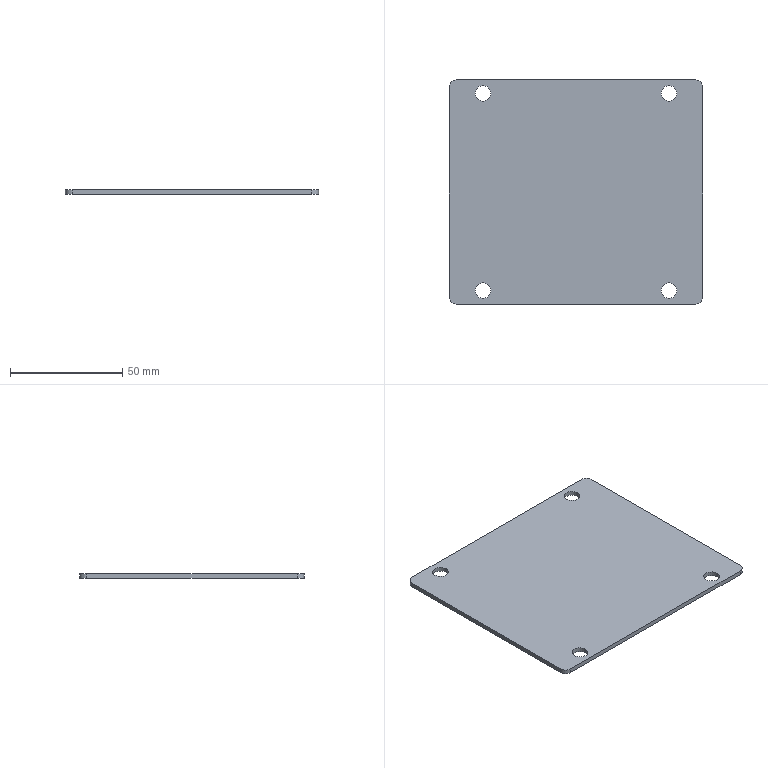Part | STEP file | Motor Cover | 1 solid | 18 faces | box 113 x 100 x 2 mm | volume 22277 mm3 | cylinder 12 | plane 6 | commonest cylinder face diameters 7 x8 6 x4
STEP:
#1=CARTESIAN_POINT('',(-20.337,41.023,-2.));
#2=VERTEX_POINT('',#1);
#3=CARTESIAN_POINT('',(-27.337,41.023,-2.));
#4=VERTEX_POINT('',#3);
#5=CARTESIAN_POINT('',(-23.837,41.023,-2.));
#6=DIRECTION('',(0.,0.,-1.));
#7=DIRECTION('',(1.,0.,0.));
#8=AXIS2_PLACEMENT_3D('',#5,#6,#7);
#9=CIRCLE('',#8,3.5);
#10=EDGE_CURVE('',#2,#4,#9,.T.);
#11=ORIENTED_EDGE('',*,*,#10,.T.);
#12=CARTESIAN_POINT('',(-27.337,41.023,0.));
#13=VERTEX_POINT('',#12);
#14=CARTESIAN_POINT('',(-27.337,41.023,-2.));
#15=DIRECTION('',(0.,0.,1.));
#16=VECTOR('',#15,1000.);
#17=LINE('',#14,#16);
#18=EDGE_CURVE('',#4,#13,#17,.T.);
#19=ORIENTED_EDGE('',*,*,#18,.T.);
#20=CARTESIAN_POINT('',(-20.337,41.023,0.));
#21=VERTEX_POINT('',#20);
#22=CARTESIAN_POINT('',(-23.837,41.023,0.));
#23=DIRECTION('',(0.,0.,-1.));
#24=DIRECTION('',(1.,0.,0.));
#25=AXIS2_PLACEMENT_3D('',#22,#23,#24);
#26=CIRCLE('',#25,3.5);
#27=EDGE_CURVE('',#21,#13,#26,.T.);
#28=ORIENTED_EDGE('',*,*,#27,.F.);
#29=CARTESIAN_POINT('',(-20.337,41.023,-2.));
#30=DIRECTION('',(0.,0.,1.));
#31=VECTOR('',#30,1000.);
#32=LINE('',#29,#31);
#33=EDGE_CURVE('',#2,#21,#32,.T.);
#34=ORIENTED_EDGE('',*,*,#33,.F.);
#35=EDGE_LOOP('',(#11,#19,#28,#34));
#36=FACE_OUTER_BOUND('',#35,.T.);
#37=CARTESIAN_POINT('',(-23.837,41.023,-2.));
#38=DIRECTION('',(0.,0.,1.));
#39=DIRECTION('',(1.,0.,0.));
#40=AXIS2_PLACEMENT_3D('',#37,#38,#39);
#41=CYLINDRICAL_SURFACE('',#40,3.5);
#42=ADVANCED_FACE('',(#36),#41,.F.);
#43=CARTESIAN_POINT('',(62.663,41.023,-2.));
#44=VERTEX_POINT('',#43);
#45=CARTESIAN_POINT('',(55.663,41.023,-2.));
#46=VERTEX_POINT('',#45);
#47=CARTESIAN_POINT('',(59.163,41.023,-2.));
#48=DIRECTION('',(0.,0.,-1.));
#49=DIRECTION('',(1.,0.,0.));
#50=AXIS2_PLACEMENT_3D('',#47,#48,#49);
#51=CIRCLE('',#50,3.5);
#52=EDGE_CURVE('',#44,#46,#51,.T.);
#53=ORIENTED_EDGE('',*,*,#52,.T.);
#54=CARTESIAN_POINT('',(55.663,41.023,0.));
#55=VERTEX_POINT('',#54);
#56=CARTESIAN_POINT('',(55.663,41.023,-2.));
#57=DIRECTION('',(0.,0.,1.));
#58=VECTOR('',#57,1000.);
#59=LINE('',#56,#58);
#60=EDGE_CURVE('',#46,#55,#59,.T.);
#61=ORIENTED_EDGE('',*,*,#60,.T.);
#62=CARTESIAN_POINT('',(62.663,41.023,0.));
#63=VERTEX_POINT('',#62);
#64=CARTESIAN_POINT('',(59.163,41.023,0.));
#65=DIRECTION('',(0.,0.,-1.));
#66=DIRECTION('',(1.,0.,0.));
#67=AXIS2_PLACEMENT_3D('',#64,#65,#66);
#68=CIRCLE('',#67,3.5);
#69=EDGE_CURVE('',#63,#55,#68,.T.);
#70=ORIENTED_EDGE('',*,*,#69,.F.);
#71=CARTESIAN_POINT('',(62.663,41.023,-2.));
#72=DIRECTION('',(0.,0.,1.));
#73=VECTOR('',#72,1000.);
#74=LINE('',#71,#73);
#75=EDGE_CURVE('',#44,#63,#74,.T.);
#76=ORIENTED_EDGE('',*,*,#75,.F.);
#77=EDGE_LOOP('',(#53,#61,#70,#76));
#78=FACE_OUTER_BOUND('',#77,.T.);
#79=CARTESIAN_POINT('',(59.163,41.023,-2.));
#80=DIRECTION('',(0.,0.,1.));
#81=DIRECTION('',(1.,0.,0.));
#82=AXIS2_PLACEMENT_3D('',#79,#80,#81);
#83=CYLINDRICAL_SURFACE('',#82,3.5);
#84=ADVANCED_FACE('',(#78),#83,.F.);
#85=CARTESIAN_POINT('',(62.663,-46.977,-2.));
#86=VERTEX_POINT('',#85);
#87=CARTESIAN_POINT('',(55.663,-46.977,-2.));
#88=VERTEX_POINT('',#87);
#89=CARTESIAN_POINT('',(59.163,-46.977,-2.));
#90=DIRECTION('',(0.,0.,-1.));
#91=DIRECTION('',(1.,0.,0.));
#92=AXIS2_PLACEMENT_3D('',#89,#90,#91);
#93=CIRCLE('',#92,3.5);
#94=EDGE_CURVE('',#86,#88,#93,.T.);
#95=ORIENTED_EDGE('',*,*,#94,.T.);
#96=CARTESIAN_POINT('',(55.663,-46.977,0.));
#97=VERTEX_POINT('',#96);
#98=CARTESIAN_POINT('',(55.663,-46.977,-2.));
#99=DIRECTION('',(0.,0.,1.));
#100=VECTOR('',#99,1000.);
#101=LINE('',#98,#100);
#102=EDGE_CURVE('',#88,#97,#101,.T.);
#103=ORIENTED_EDGE('',*,*,#102,.T.);
#104=CARTESIAN_POINT('',(62.663,-46.977,0.));
#105=VERTEX_POINT('',#104);
#106=CARTESIAN_POINT('',(59.163,-46.977,0.));
#107=DIRECTION('',(0.,0.,-1.));
#108=DIRECTION('',(1.,0.,0.));
#109=AXIS2_PLACEMENT_3D('',#106,#107,#108);
#110=CIRCLE('',#109,3.5);
#111=EDGE_CURVE('',#105,#97,#110,.T.);
#112=ORIENTED_EDGE('',*,*,#111,.F.);
#113=CARTESIAN_POINT('',(62.663,-46.977,-2.));
#114=DIRECTION('',(0.,0.,1.));
#115=VECTOR('',#114,1000.);
#116=LINE('',#113,#115);
#117=EDGE_CURVE('',#86,#105,#116,.T.);
#118=ORIENTED_EDGE('',*,*,#117,.F.);
#119=EDGE_LOOP('',(#95,#103,#112,#118));
#120=FACE_OUTER_BOUND('',#119,.T.);
#121=CARTESIAN_POINT('',(59.163,-46.977,-2.));
#122=DIRECTION('',(0.,0.,1.));
#123=DIRECTION('',(1.,0.,0.));
#124=AXIS2_PLACEMENT_3D('',#121,#122,#123);
#125=CYLINDRICAL_SURFACE('',#124,3.5);
#126=ADVANCED_FACE('',(#120),#125,.F.);
#127=CARTESIAN_POINT('',(-20.337,-46.977,-2.));
#128=VERTEX_POINT('',#127);
#129=CARTESIAN_POINT('',(-27.337,-46.977,-2.));
#130=VERTEX_POINT('',#129);
#131=CARTESIAN_POINT('',(-23.837,-46.977,-2.));
#132=DIRECTION('',(0.,0.,-1.));
#133=DIRECTION('',(1.,0.,0.));
#134=AXIS2_PLACEMENT_3D('',#131,#132,#133);
#135=CIRCLE('',#134,3.5);
#136=EDGE_CURVE('',#128,#130,#135,.T.);
#137=ORIENTED_EDGE('',*,*,#136,.T.);
#138=CARTESIAN_POINT('',(-27.337,-46.977,0.));
#139=VERTEX_POINT('',#138);
#140=CARTESIAN_POINT('',(-27.337,-46.977,-2.));
#141=DIRECTION('',(0.,0.,1.));
#142=VECTOR('',#141,1000.);
#143=LINE('',#140,#142);
#144=EDGE_CURVE('',#130,#139,#143,.T.);
#145=ORIENTED_EDGE('',*,*,#144,.T.);
#146=CARTESIAN_POINT('',(-20.337,-46.977,0.));
#147=VERTEX_POINT('',#146);
#148=CARTESIAN_POINT('',(-23.837,-46.977,0.));
#149=DIRECTION('',(0.,0.,-1.));
#150=DIRECTION('',(1.,0.,0.));
#151=AXIS2_PLACEMENT_3D('',#148,#149,#150);
#152=CIRCLE('',#151,3.5);
#153=EDGE_CURVE('',#147,#139,#152,.T.);
#154=ORIENTED_EDGE('',*,*,#153,.F.);
#155=CARTESIAN_POINT('',(-20.337,-46.977,-2.));
#156=DIRECTION('',(0.,0.,1.));
#157=VECTOR('',#156,1000.);
#158=LINE('',#155,#157);
#159=EDGE_CURVE('',#128,#147,#158,.T.);
#160=ORIENTED_EDGE('',*,*,#159,.F.);
#161=EDGE_LOOP('',(#137,#145,#154,#160));
#162=FACE_OUTER_BOUND('',#161,.T.);
#163=CARTESIAN_POINT('',(-23.837,-46.977,-2.));
#164=DIRECTION('',(0.,0.,1.));
#165=DIRECTION('',(1.,0.,0.));
#166=AXIS2_PLACEMENT_3D('',#163,#164,#165);
#167=CYLINDRICAL_SURFACE('',#166,3.5);
#168=ADVANCED_FACE('',(#162),#167,.F.);
#169=CARTESIAN_POINT('',(74.163,44.023,-2.));
#170=VERTEX_POINT('',#169);
#171=CARTESIAN_POINT('',(71.163,47.023,-2.));
#172=VERTEX_POINT('',#171);
#173=CARTESIAN_POINT('',(71.163,44.023,-2.));
#174=DIRECTION('',(0.,0.,1.));
#175=DIRECTION('',(1.,0.,0.));
#176=AXIS2_PLACEMENT_3D('',#173,#174,#175);
#177=CIRCLE('',#176,3.);
#178=EDGE_CURVE('',#170,#172,#177,.T.);
#179=ORIENTED_EDGE('',*,*,#178,.F.);
#180=CARTESIAN_POINT('',(74.163,-49.977,-2.));
#181=VERTEX_POINT('',#180);
#182=CARTESIAN_POINT('',(74.163,0.,-2.));
#183=DIRECTION('',(0.,1.,0.));
#184=VECTOR('',#183,1000.);
#185=LINE('',#182,#184);
#186=EDGE_CURVE('',#181,#170,#185,.T.);
#187=ORIENTED_EDGE('',*,*,#186,.F.);
#188=CARTESIAN_POINT('',(71.163,-52.977,-2.));
#189=VERTEX_POINT('',#188);
#190=CARTESIAN_POINT('',(71.163,-49.977,-2.));
#191=DIRECTION('',(0.,0.,1.));
#192=DIRECTION('',(1.,0.,0.));
#193=AXIS2_PLACEMENT_3D('',#190,#191,#192);
#194=CIRCLE('',#193,3.);
#195=EDGE_CURVE('',#189,#181,#194,.T.);
#196=ORIENTED_EDGE('',*,*,#195,.F.);
#197=CARTESIAN_POINT('',(-35.837,-52.977,-2.));
#198=VERTEX_POINT('',#197);
#199=CARTESIAN_POINT('',(0.,-52.977,-2.));
#200=DIRECTION('',(1.,0.,0.));
#201=VECTOR('',#200,1000.);
#202=LINE('',#199,#201);
#203=EDGE_CURVE('',#198,#189,#202,.T.);
#204=ORIENTED_EDGE('',*,*,#203,.F.);
#205=CARTESIAN_POINT('',(-38.837,-49.977,-2.));
#206=VERTEX_POINT('',#205);
#207=CARTESIAN_POINT('',(-35.837,-49.977,-2.));
#208=DIRECTION('',(0.,0.,1.));
#209=DIRECTION('',(1.,0.,0.));
#210=AXIS2_PLACEMENT_3D('',#207,#208,#209);
#211=CIRCLE('',#210,3.);
#212=EDGE_CURVE('',#206,#198,#211,.T.);
#213=ORIENTED_EDGE('',*,*,#212,.F.);
#214=CARTESIAN_POINT('',(-38.837,44.023,-2.));
#215=VERTEX_POINT('',#214);
#216=CARTESIAN_POINT('',(-38.837,0.,-2.));
#217=DIRECTION('',(0.,-1.,0.));
#218=VECTOR('',#217,1000.);
#219=LINE('',#216,#218);
#220=EDGE_CURVE('',#215,#206,#219,.T.);
#221=ORIENTED_EDGE('',*,*,#220,.F.);
#222=CARTESIAN_POINT('',(-35.837,47.023,-2.));
#223=VERTEX_POINT('',#222);
#224=CARTESIAN_POINT('',(-35.837,44.023,-2.));
#225=DIRECTION('',(0.,0.,1.));
#226=DIRECTION('',(1.,0.,0.));
#227=AXIS2_PLACEMENT_3D('',#224,#225,#226);
#228=CIRCLE('',#227,3.);
#229=EDGE_CURVE('',#223,#215,#228,.T.);
#230=ORIENTED_EDGE('',*,*,#229,.F.);
#231=CARTESIAN_POINT('',(0.,47.023,-2.));
#232=DIRECTION('',(-1.,0.,0.));
#233=VECTOR('',#232,1000.);
#234=LINE('',#231,#233);
#235=EDGE_CURVE('',#172,#223,#234,.T.);
#236=ORIENTED_EDGE('',*,*,#235,.F.);
#237=EDGE_LOOP('',(#179,#187,#196,#204,#213,#221,#230,#236));
#238=FACE_OUTER_BOUND('',#237,.T.);
#239=ORIENTED_EDGE('',*,*,#10,.F.);
#240=CARTESIAN_POINT('',(-23.837,41.023,-2.));
#241=DIRECTION('',(0.,0.,-1.));
#242=DIRECTION('',(1.,0.,0.));
#243=AXIS2_PLACEMENT_3D('',#240,#241,#242);
#244=CIRCLE('',#243,3.5);
#245=EDGE_CURVE('',#4,#2,#244,.T.);
#246=ORIENTED_EDGE('',*,*,#245,.F.);
#247=EDGE_LOOP('',(#239,#246));
#248=FACE_BOUND('',#247,.T.);
#249=ORIENTED_EDGE('',*,*,#52,.F.);
#250=CARTESIAN_POINT('',(59.163,41.023,-2.));
#251=DIRECTION('',(0.,0.,-1.));
#252=DIRECTION('',(1.,0.,0.));
#253=AXIS2_PLACEMENT_3D('',#250,#251,#252);
#254=CIRCLE('',#253,3.5);
#255=EDGE_CURVE('',#46,#44,#254,.T.);
#256=ORIENTED_EDGE('',*,*,#255,.F.);
#257=EDGE_LOOP('',(#249,#256));
#258=FACE_BOUND('',#257,.T.);
#259=ORIENTED_EDGE('',*,*,#94,.F.);
#260=CARTESIAN_POINT('',(59.163,-46.977,-2.));
#261=DIRECTION('',(0.,0.,-1.));
#262=DIRECTION('',(1.,0.,0.));
#263=AXIS2_PLACEMENT_3D('',#260,#261,#262);
#264=CIRCLE('',#263,3.5);
#265=EDGE_CURVE('',#88,#86,#264,.T.);
#266=ORIENTED_EDGE('',*,*,#265,.F.);
#267=EDGE_LOOP('',(#259,#266));
#268=FACE_BOUND('',#267,.T.);
#269=ORIENTED_EDGE('',*,*,#136,.F.);
#270=CARTESIAN_POINT('',(-23.837,-46.977,-2.));
#271=DIRECTION('',(0.,0.,-1.));
#272=DIRECTION('',(1.,0.,0.));
#273=AXIS2_PLACEMENT_3D('',#270,#271,#272);
#274=CIRCLE('',#273,3.5);
#275=EDGE_CURVE('',#130,#128,#274,.T.);
#276=ORIENTED_EDGE('',*,*,#275,.F.);
#277=EDGE_LOOP('',(#269,#276));
#278=FACE_BOUND('',#277,.T.);
#279=CARTESIAN_POINT('',(0.,0.,-2.));
#280=DIRECTION('',(0.,0.,1.));
#281=DIRECTION('',(1.,0.,0.));
#282=AXIS2_PLACEMENT_3D('',#279,#280,#281);
#283=PLANE('',#282);
#284=ADVANCED_FACE('',(#238,#248,#258,#268,#278),#283,.F.);
#285=ORIENTED_EDGE('',*,*,#235,.T.);
#286=CARTESIAN_POINT('',(-35.837,47.023,0.));
#287=VERTEX_POINT('',#286);
#288=CARTESIAN_POINT('',(-35.837,47.023,-2.));
#289=DIRECTION('',(0.,0.,1.));
#290=VECTOR('',#289,1000.);
#291=LINE('',#288,#290);
#292=EDGE_CURVE('',#223,#287,#291,.T.);
#293=ORIENTED_EDGE('',*,*,#292,.T.);
#294=CARTESIAN_POINT('',(71.163,47.023,0.));
#295=VERTEX_POINT('',#294);
#296=CARTESIAN_POINT('',(-38.837,47.023,0.));
#297=DIRECTION('',(1.,0.,0.));
#298=VECTOR('',#297,1000.);
#299=LINE('',#296,#298);
#300=EDGE_CURVE('',#287,#295,#299,.T.);
#301=ORIENTED_EDGE('',*,*,#300,.T.);
#302=CARTESIAN_POINT('',(71.163,47.023,-2.));
#303=DIRECTION('',(0.,0.,-1.));
#304=VECTOR('',#303,1000.);
#305=LINE('',#302,#304);
#306=EDGE_CURVE('',#295,#172,#305,.T.);
#307=ORIENTED_EDGE('',*,*,#306,.T.);
#308=EDGE_LOOP('',(#285,#293,#301,#307));
#309=FACE_OUTER_BOUND('',#308,.T.);
#310=CARTESIAN_POINT('',(-38.837,47.023,-2.));
#311=DIRECTION('',(0.,1.,0.));
#312=DIRECTION('',(0.,0.,1.));
#313=AXIS2_PLACEMENT_3D('',#310,#311,#312);
#314=PLANE('',#313);
#315=ADVANCED_FACE('',(#309),#314,.T.);
#316=CARTESIAN_POINT('',(74.163,44.023,0.));
#317=VERTEX_POINT('',#316);
#318=CARTESIAN_POINT('',(71.163,44.023,0.));
#319=DIRECTION('',(0.,0.,-1.));
#320=DIRECTION('',(1.,0.,0.));
#321=AXIS2_PLACEMENT_3D('',#318,#319,#320);
#322=CIRCLE('',#321,3.);
#323=EDGE_CURVE('',#295,#317,#322,.T.);
#324=ORIENTED_EDGE('',*,*,#323,.T.);
#325=CARTESIAN_POINT('',(74.163,44.023,-2.));
#326=DIRECTION('',(0.,0.,-1.));
#327=VECTOR('',#326,1000.);
#328=LINE('',#325,#327);
#329=EDGE_CURVE('',#317,#170,#328,.T.);
#330=ORIENTED_EDGE('',*,*,#329,.T.);
#331=ORIENTED_EDGE('',*,*,#178,.T.);
#332=ORIENTED_EDGE('',*,*,#306,.F.);
#333=EDGE_LOOP('',(#324,#330,#331,#332));
#334=FACE_OUTER_BOUND('',#333,.T.);
#335=CARTESIAN_POINT('',(71.163,44.023,-2.));
#336=DIRECTION('',(0.,0.,1.));
#337=DIRECTION('',(1.,0.,0.));
#338=AXIS2_PLACEMENT_3D('',#335,#336,#337);
#339=CYLINDRICAL_SURFACE('',#338,3.);
#340=ADVANCED_FACE('',(#334),#339,.T.);
#341=CARTESIAN_POINT('',(74.163,-49.977,0.));
#342=VERTEX_POINT('',#341);
#343=CARTESIAN_POINT('',(74.163,47.023,0.));
#344=DIRECTION('',(0.,-1.,0.));
#345=VECTOR('',#344,1000.);
#346=LINE('',#343,#345);
#347=EDGE_CURVE('',#317,#342,#346,.T.);
#348=ORIENTED_EDGE('',*,*,#347,.T.);
#349=CARTESIAN_POINT('',(74.163,-49.977,-2.));
#350=DIRECTION('',(0.,0.,-1.));
#351=VECTOR('',#350,1000.);
#352=LINE('',#349,#351);
#353=EDGE_CURVE('',#342,#181,#352,.T.);
#354=ORIENTED_EDGE('',*,*,#353,.T.);
#355=ORIENTED_EDGE('',*,*,#186,.T.);
#356=ORIENTED_EDGE('',*,*,#329,.F.);
#357=EDGE_LOOP('',(#348,#354,#355,#356));
#358=FACE_OUTER_BOUND('',#357,.T.);
#359=CARTESIAN_POINT('',(74.163,47.023,-2.));
#360=DIRECTION('',(1.,0.,0.));
#361=DIRECTION('',(0.,0.,-1.));
#362=AXIS2_PLACEMENT_3D('',#359,#360,#361);
#363=PLANE('',#362);
#364=ADVANCED_FACE('',(#358),#363,.T.);
#365=CARTESIAN_POINT('',(71.163,-52.977,0.));
#366=VERTEX_POINT('',#365);
#367=CARTESIAN_POINT('',(71.163,-49.977,0.));
#368=DIRECTION('',(0.,0.,-1.));
#369=DIRECTION('',(1.,0.,0.));
#370=AXIS2_PLACEMENT_3D('',#367,#368,#369);
#371=CIRCLE('',#370,3.);
#372=EDGE_CURVE('',#342,#366,#371,.T.);
#373=ORIENTED_EDGE('',*,*,#372,.T.);
#374=CARTESIAN_POINT('',(71.163,-52.977,-2.));
#375=DIRECTION('',(0.,0.,-1.));
#376=VECTOR('',#375,1000.);
#377=LINE('',#374,#376);
#378=EDGE_CURVE('',#366,#189,#377,.T.);
#379=ORIENTED_EDGE('',*,*,#378,.T.);
#380=ORIENTED_EDGE('',*,*,#195,.T.);
#381=ORIENTED_EDGE('',*,*,#353,.F.);
#382=EDGE_LOOP('',(#373,#379,#380,#381));
#383=FACE_OUTER_BOUND('',#382,.T.);
#384=CARTESIAN_POINT('',(71.163,-49.977,-2.));
#385=DIRECTION('',(0.,0.,1.));
#386=DIRECTION('',(1.,0.,0.));
#387=AXIS2_PLACEMENT_3D('',#384,#385,#386);
#388=CYLINDRICAL_SURFACE('',#387,3.);
#389=ADVANCED_FACE('',(#383),#388,.T.);
#390=CARTESIAN_POINT('',(-35.837,-52.977,0.));
#391=VERTEX_POINT('',#390);
#392=CARTESIAN_POINT('',(-38.837,-52.977,0.));
#393=DIRECTION('',(-1.,0.,0.));
#394=VECTOR('',#393,1000.);
#395=LINE('',#392,#394);
#396=EDGE_CURVE('',#366,#391,#395,.T.);
#397=ORIENTED_EDGE('',*,*,#396,.T.);
#398=CARTESIAN_POINT('',(-35.837,-52.977,-2.));
#399=DIRECTION('',(0.,0.,-1.));
#400=VECTOR('',#399,1000.);
#401=LINE('',#398,#400);
#402=EDGE_CURVE('',#391,#198,#401,.T.);
#403=ORIENTED_EDGE('',*,*,#402,.T.);
#404=ORIENTED_EDGE('',*,*,#203,.T.);
#405=ORIENTED_EDGE('',*,*,#378,.F.);
#406=EDGE_LOOP('',(#397,#403,#404,#405));
#407=FACE_OUTER_BOUND('',#406,.T.);
#408=CARTESIAN_POINT('',(-38.837,-52.977,-2.));
#409=DIRECTION('',(0.,-1.,0.));
#410=DIRECTION('',(0.,0.,-1.));
#411=AXIS2_PLACEMENT_3D('',#408,#409,#410);
#412=PLANE('',#411);
#413=ADVANCED_FACE('',(#407),#412,.T.);
#414=CARTESIAN_POINT('',(-38.837,-49.977,0.));
#415=VERTEX_POINT('',#414);
#416=CARTESIAN_POINT('',(-35.837,-49.977,0.));
#417=DIRECTION('',(0.,0.,-1.));
#418=DIRECTION('',(1.,0.,0.));
#419=AXIS2_PLACEMENT_3D('',#416,#417,#418);
#420=CIRCLE('',#419,3.);
#421=EDGE_CURVE('',#391,#415,#420,.T.);
#422=ORIENTED_EDGE('',*,*,#421,.T.);
#423=CARTESIAN_POINT('',(-38.837,-49.977,-2.));
#424=DIRECTION('',(0.,0.,-1.));
#425=VECTOR('',#424,1000.);
#426=LINE('',#423,#425);
#427=EDGE_CURVE('',#415,#206,#426,.T.);
#428=ORIENTED_EDGE('',*,*,#427,.T.);
#429=ORIENTED_EDGE('',*,*,#212,.T.);
#430=ORIENTED_EDGE('',*,*,#402,.F.);
#431=EDGE_LOOP('',(#422,#428,#429,#430));
#432=FACE_OUTER_BOUND('',#431,.T.);
#433=CARTESIAN_POINT('',(-35.837,-49.977,-2.));
#434=DIRECTION('',(0.,0.,1.));
#435=DIRECTION('',(1.,0.,0.));
#436=AXIS2_PLACEMENT_3D('',#433,#434,#435);
#437=CYLINDRICAL_SURFACE('',#436,3.);
#438=ADVANCED_FACE('',(#432),#437,.T.);
#439=CARTESIAN_POINT('',(-38.837,44.023,0.));
#440=VERTEX_POINT('',#439);
#441=CARTESIAN_POINT('',(-38.837,47.023,0.));
#442=DIRECTION('',(0.,1.,0.));
#443=VECTOR('',#442,1000.);
#444=LINE('',#441,#443);
#445=EDGE_CURVE('',#415,#440,#444,.T.);
#446=ORIENTED_EDGE('',*,*,#445,.T.);
#447=CARTESIAN_POINT('',(-38.837,44.023,-2.));
#448=DIRECTION('',(0.,0.,-1.));
#449=VECTOR('',#448,1000.);
#450=LINE('',#447,#449);
#451=EDGE_CURVE('',#440,#215,#450,.T.);
#452=ORIENTED_EDGE('',*,*,#451,.T.);
#453=ORIENTED_EDGE('',*,*,#220,.T.);
#454=ORIENTED_EDGE('',*,*,#427,.F.);
#455=EDGE_LOOP('',(#446,#452,#453,#454));
#456=FACE_OUTER_BOUND('',#455,.T.);
#457=CARTESIAN_POINT('',(-38.837,47.023,-2.));
#458=DIRECTION('',(-1.,0.,0.));
#459=DIRECTION('',(0.,0.,1.));
#460=AXIS2_PLACEMENT_3D('',#457,#458,#459);
#461=PLANE('',#460);
#462=ADVANCED_FACE('',(#456),#461,.T.);
#463=CARTESIAN_POINT('',(-35.837,44.023,0.));
#464=DIRECTION('',(0.,0.,-1.));
#465=DIRECTION('',(1.,0.,0.));
#466=AXIS2_PLACEMENT_3D('',#463,#464,#465);
#467=CIRCLE('',#466,3.);
#468=EDGE_CURVE('',#440,#287,#467,.T.);
#469=ORIENTED_EDGE('',*,*,#468,.T.);
#470=ORIENTED_EDGE('',*,*,#292,.F.);
#471=ORIENTED_EDGE('',*,*,#229,.T.);
#472=ORIENTED_EDGE('',*,*,#451,.F.);
#473=EDGE_LOOP('',(#469,#470,#471,#472));
#474=FACE_OUTER_BOUND('',#473,.T.);
#475=CARTESIAN_POINT('',(-35.837,44.023,-2.));
#476=DIRECTION('',(0.,0.,1.));
#477=DIRECTION('',(1.,0.,0.));
#478=AXIS2_PLACEMENT_3D('',#475,#476,#477);
#479=CYLINDRICAL_SURFACE('',#478,3.);
#480=ADVANCED_FACE('',(#474),#479,.T.);
#481=ORIENTED_EDGE('',*,*,#18,.F.);
#482=ORIENTED_EDGE('',*,*,#245,.T.);
#483=ORIENTED_EDGE('',*,*,#33,.T.);
#484=CARTESIAN_POINT('',(-23.837,41.023,0.));
#485=DIRECTION('',(0.,0.,-1.));
#486=DIRECTION('',(1.,0.,0.));
#487=AXIS2_PLACEMENT_3D('',#484,#485,#486);
#488=CIRCLE('',#487,3.5);
#489=EDGE_CURVE('',#13,#21,#488,.T.);
#490=ORIENTED_EDGE('',*,*,#489,.F.);
#491=EDGE_LOOP('',(#481,#482,#483,#490));
#492=FACE_OUTER_BOUND('',#491,.T.);
#493=CARTESIAN_POINT('',(-23.837,41.023,-2.));
#494=DIRECTION('',(0.,0.,1.));
#495=DIRECTION('',(1.,0.,0.));
#496=AXIS2_PLACEMENT_3D('',#493,#494,#495);
#497=CYLINDRICAL_SURFACE('',#496,3.5);
#498=ADVANCED_FACE('',(#492),#497,.F.);
#499=ORIENTED_EDGE('',*,*,#60,.F.);
#500=ORIENTED_EDGE('',*,*,#255,.T.);
#501=ORIENTED_EDGE('',*,*,#75,.T.);
#502=CARTESIAN_POINT('',(59.163,41.023,0.));
#503=DIRECTION('',(0.,0.,-1.));
#504=DIRECTION('',(1.,0.,0.));
#505=AXIS2_PLACEMENT_3D('',#502,#503,#504);
#506=CIRCLE('',#505,3.5);
#507=EDGE_CURVE('',#55,#63,#506,.T.);
#508=ORIENTED_EDGE('',*,*,#507,.F.);
#509=EDGE_LOOP('',(#499,#500,#501,#508));
#510=FACE_OUTER_BOUND('',#509,.T.);
#511=CARTESIAN_POINT('',(59.163,41.023,-2.));
#512=DIRECTION('',(0.,0.,1.));
#513=DIRECTION('',(1.,0.,0.));
#514=AXIS2_PLACEMENT_3D('',#511,#512,#513);
#515=CYLINDRICAL_SURFACE('',#514,3.5);
#516=ADVANCED_FACE('',(#510),#515,.F.);
#517=ORIENTED_EDGE('',*,*,#102,.F.);
#518=ORIENTED_EDGE('',*,*,#265,.T.);
#519=ORIENTED_EDGE('',*,*,#117,.T.);
#520=CARTESIAN_POINT('',(59.163,-46.977,0.));
#521=DIRECTION('',(0.,0.,-1.));
#522=DIRECTION('',(1.,0.,0.));
#523=AXIS2_PLACEMENT_3D('',#520,#521,#522);
#524=CIRCLE('',#523,3.5);
#525=EDGE_CURVE('',#97,#105,#524,.T.);
#526=ORIENTED_EDGE('',*,*,#525,.F.);
#527=EDGE_LOOP('',(#517,#518,#519,#526));
#528=FACE_OUTER_BOUND('',#527,.T.);
#529=CARTESIAN_POINT('',(59.163,-46.977,-2.));
#530=DIRECTION('',(0.,0.,1.));
#531=DIRECTION('',(1.,0.,0.));
#532=AXIS2_PLACEMENT_3D('',#529,#530,#531);
#533=CYLINDRICAL_SURFACE('',#532,3.5);
#534=ADVANCED_FACE('',(#528),#533,.F.);
#535=ORIENTED_EDGE('',*,*,#144,.F.);
#536=ORIENTED_EDGE('',*,*,#275,.T.);
#537=ORIENTED_EDGE('',*,*,#159,.T.);
#538=CARTESIAN_POINT('',(-23.837,-46.977,0.));
#539=DIRECTION('',(0.,0.,-1.));
#540=DIRECTION('',(1.,0.,0.));
#541=AXIS2_PLACEMENT_3D('',#538,#539,#540);
#542=CIRCLE('',#541,3.5);
#543=EDGE_CURVE('',#139,#147,#542,.T.);
#544=ORIENTED_EDGE('',*,*,#543,.F.);
#545=EDGE_LOOP('',(#535,#536,#537,#544));
#546=FACE_OUTER_BOUND('',#545,.T.);
#547=CARTESIAN_POINT('',(-23.837,-46.977,-2.));
#548=DIRECTION('',(0.,0.,1.));
#549=DIRECTION('',(1.,0.,0.));
#550=AXIS2_PLACEMENT_3D('',#547,#548,#549);
#551=CYLINDRICAL_SURFACE('',#550,3.5);
#552=ADVANCED_FACE('',(#546),#551,.F.);
#553=ORIENTED_EDGE('',*,*,#396,.F.);
#554=ORIENTED_EDGE('',*,*,#372,.F.);
#555=ORIENTED_EDGE('',*,*,#347,.F.);
#556=ORIENTED_EDGE('',*,*,#323,.F.);
#557=ORIENTED_EDGE('',*,*,#300,.F.);
#558=ORIENTED_EDGE('',*,*,#468,.F.);
#559=ORIENTED_EDGE('',*,*,#445,.F.);
#560=ORIENTED_EDGE('',*,*,#421,.F.);
#561=EDGE_LOOP('',(#553,#554,#555,#556,#557,#558,#559,#560));
#562=FACE_OUTER_BOUND('',#561,.T.);
#563=ORIENTED_EDGE('',*,*,#27,.T.);
#564=ORIENTED_EDGE('',*,*,#489,.T.);
#565=EDGE_LOOP('',(#563,#564));
#566=FACE_BOUND('',#565,.T.);
#567=ORIENTED_EDGE('',*,*,#69,.T.);
#568=ORIENTED_EDGE('',*,*,#507,.T.);
#569=EDGE_LOOP('',(#567,#568));
#570=FACE_BOUND('',#569,.T.);
#571=ORIENTED_EDGE('',*,*,#111,.T.);
#572=ORIENTED_EDGE('',*,*,#525,.T.);
#573=EDGE_LOOP('',(#571,#572));
#574=FACE_BOUND('',#573,.T.);
#575=ORIENTED_EDGE('',*,*,#153,.T.);
#576=ORIENTED_EDGE('',*,*,#543,.T.);
#577=EDGE_LOOP('',(#575,#576));
#578=FACE_BOUND('',#577,.T.);
#579=CARTESIAN_POINT('',(0.,0.,0.));
#580=DIRECTION('',(0.,0.,1.));
#581=DIRECTION('',(1.,0.,0.));
#582=AXIS2_PLACEMENT_3D('',#579,#580,#581);
#583=PLANE('',#582);
#584=ADVANCED_FACE('',(#562,#566,#570,#574,#578),#583,.T.);
#585=CLOSED_SHELL('',(#42,#84,#126,#168,#284,#315,#340,#364,#389,#413,#438,#462,#480,#498,#516,#534,#552,#584));
#586=MANIFOLD_SOLID_BREP('',#585);
#587=CARTESIAN_POINT('',(0.,0.,0.));
#588=DIRECTION('',(0.,0.,1.));
#589=DIRECTION('',(1.,0.,0.));
#590=AXIS2_PLACEMENT_3D('',#587,#588,#589);
#591=(LENGTH_UNIT()NAMED_UNIT(*)SI_UNIT(.MILLI.,.METRE.));
#592=UNCERTAINTY_MEASURE_WITH_UNIT(LENGTH_MEASURE(0.00001),#591,'','');
#593=(NAMED_UNIT(*)PLANE_ANGLE_UNIT()SI_UNIT($,.RADIAN.));
#594=(NAMED_UNIT(*)SI_UNIT($,.STERADIAN.)SOLID_ANGLE_UNIT());
#595=(GEOMETRIC_REPRESENTATION_CONTEXT(3)GLOBAL_UNCERTAINTY_ASSIGNED_CONTEXT((#592))GLOBAL_UNIT_ASSIGNED_CONTEXT((#591,#593,#594))REPRESENTATION_CONTEXT('',''));
#596=ADVANCED_BREP_SHAPE_REPRESENTATION('',(#586,#590),#595);